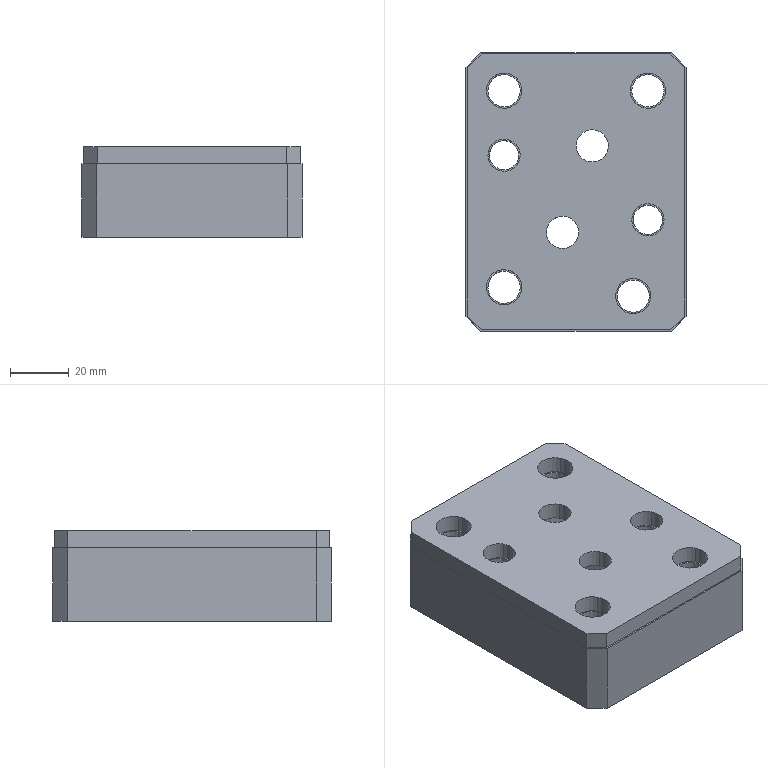Part | CATIA | 2 solids | 68 faces | box 75 x 95 x 30.8 mm | volume 163916 mm3 | cylinder 40 | plane 28 | commonest cylinder face diameters 11 x16 12 x8 18 x8 10 x6 6 x2